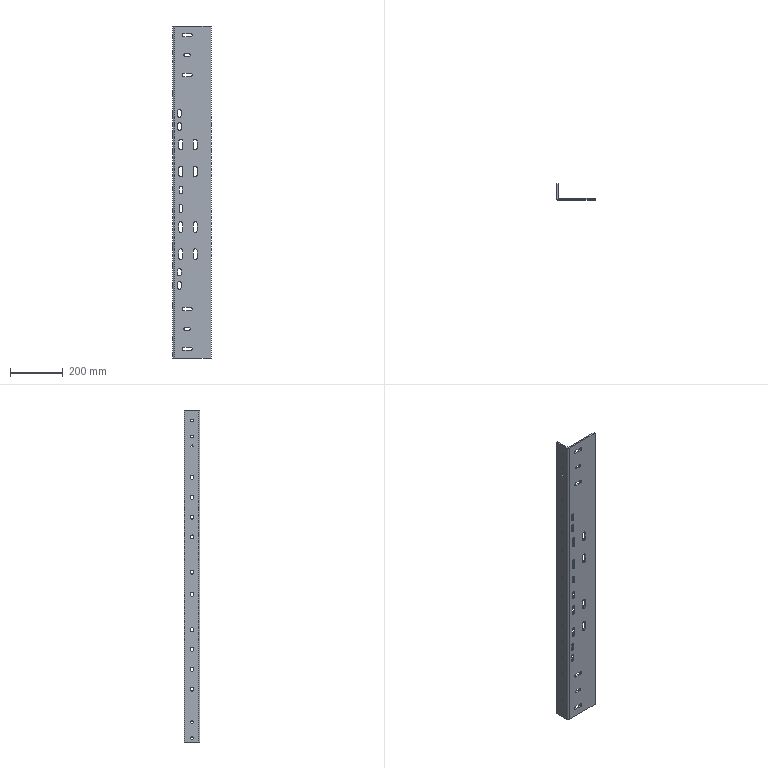Part | 1 solid | 139 faces | box 145 x 60 x 1255 mm | volume 1423811 mm3 | cylinder 84 | plane 55 | commonest cylinder face diameters 13 x26 14 x24 15 x20 10 x8 11 x4 0.4 x1